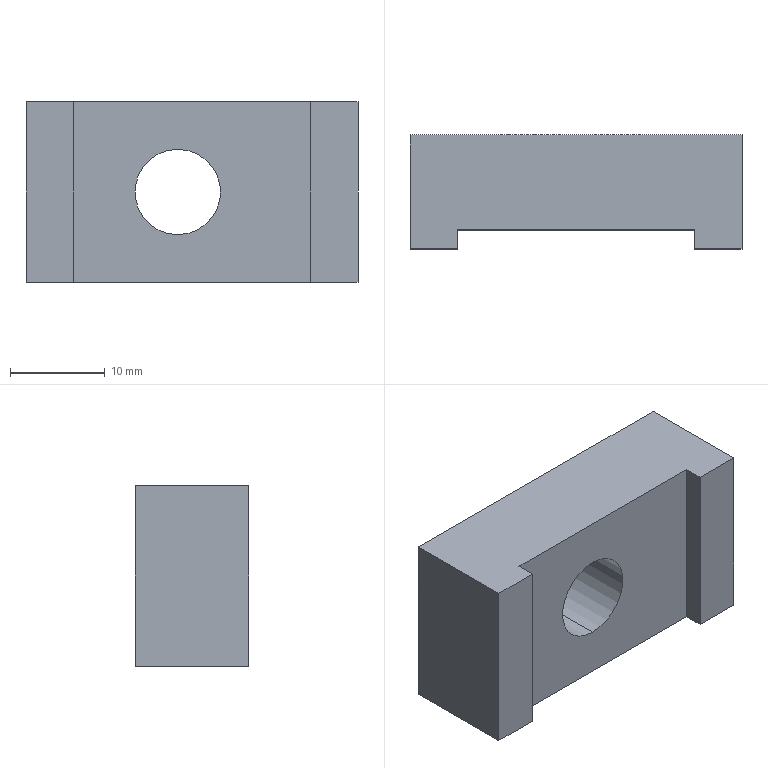Part | STEP file | OP10-023_clamp | 1 solid | 12 faces | box 35 x 12 x 19 mm | volume 6394 mm3 | plane 10 | cylinder 2 | commonest cylinder face diameters 9 x2
STEP:
#1=CARTESIAN_POINT('',(0.,0.,0.));
#2=DIRECTION('',(0.,0.,1.));
#3=DIRECTION('',(1.,0.,0.));
#4=AXIS2_PLACEMENT_3D('',#1,#2,#3);
#5=CARTESIAN_POINT('',(-1.5,-4.,14.));
#6=VERTEX_POINT('',#5);
#7=CARTESIAN_POINT('',(-1.5,6.,14.));
#8=VERTEX_POINT('',#7);
#9=CARTESIAN_POINT('',(-1.5,-13.,14.));
#10=DIRECTION('',(0.,1.,0.));
#11=VECTOR('',#10,1.);
#12=LINE('',#9,#11);
#13=CARTESIAN_POINT('',(-1.5,-13.,9.5));
#14=DIRECTION('',(0.,1.,0.));
#15=DIRECTION('',(0.,0.,1.));
#16=AXIS2_PLACEMENT_3D('',#13,#14,#15);
#17=CYLINDRICAL_SURFACE('',#16,4.5);
#18=CARTESIAN_POINT('',(6.283,0.));
#19=DIRECTION('',(0.,1.));
#20=VECTOR('',#19,1.);
#21=LINE('',#18,#20);
#22=(GEOMETRIC_REPRESENTATION_CONTEXT(2)PARAMETRIC_REPRESENTATION_CONTEXT()REPRESENTATION_CONTEXT('',''));
#23=DEFINITIONAL_REPRESENTATION('',(#21),#22);
#24=PCURVE('',#17,#23);
#25=CARTESIAN_POINT('',(-1.5,-13.,9.5));
#26=DIRECTION('',(0.,1.,0.));
#27=DIRECTION('',(0.,0.,1.));
#28=AXIS2_PLACEMENT_3D('',#25,#26,#27);
#29=CYLINDRICAL_SURFACE('',#28,4.5);
#30=CARTESIAN_POINT('',(0.,0.));
#31=DIRECTION('',(0.,1.));
#32=VECTOR('',#31,1.);
#33=LINE('',#30,#32);
#34=(GEOMETRIC_REPRESENTATION_CONTEXT(2)PARAMETRIC_REPRESENTATION_CONTEXT()REPRESENTATION_CONTEXT('',''));
#35=DEFINITIONAL_REPRESENTATION('',(#33),#34);
#36=PCURVE('',#29,#35);
#37=SURFACE_CURVE('',#12,(#24,#36),.PCURVE_S1.);
#38=EDGE_CURVE('',#6,#8,#37,.T.);
#39=ORIENTED_EDGE('',*,*,#38,.T.);
#40=CARTESIAN_POINT('',(-1.5,6.,5.));
#41=VERTEX_POINT('',#40);
#42=CARTESIAN_POINT('',(-1.5,6.,9.5));
#43=DIRECTION('',(0.,1.,0.));
#44=DIRECTION('',(0.,0.,1.));
#45=AXIS2_PLACEMENT_3D('',#42,#43,#44);
#46=CIRCLE('',#45,4.5);
#47=CARTESIAN_POINT('',(0.,19.));
#48=DIRECTION('',(1.,0.));
#49=VECTOR('',#48,1.);
#50=LINE('',#47,#49);
#51=(GEOMETRIC_REPRESENTATION_CONTEXT(2)PARAMETRIC_REPRESENTATION_CONTEXT()REPRESENTATION_CONTEXT('',''));
#52=DEFINITIONAL_REPRESENTATION('',(#50),#51);
#53=PCURVE('',#17,#52);
#54=CARTESIAN_POINT('',(-17.5,6.,19.));
#55=DIRECTION('',(0.,-1.,0.));
#56=DIRECTION('',(0.,0.,-1.));
#57=AXIS2_PLACEMENT_3D('',#54,#55,#56);
#58=PLANE('',#57);
#59=CARTESIAN_POINT('',(5.,16.));
#60=CARTESIAN_POINT('',(5.,23.794));
#61=CARTESIAN_POINT('',(11.75,19.897));
#62=CARTESIAN_POINT('',(18.5,16.));
#63=CARTESIAN_POINT('',(11.75,12.103));
#64=CARTESIAN_POINT('',(5.,8.206));
#65=CARTESIAN_POINT('',(5.,16.));
#66=(BOUNDED_CURVE()B_SPLINE_CURVE(2,(#59,#60,#61,#62,#63,#64,#65),.UNSPECIFIED.,.T.,.F.)B_SPLINE_CURVE_WITH_KNOTS((1,2,2,2,2,1),(-2.094,0.,2.094,4.189,6.283,8.378),.UNSPECIFIED.)CURVE()GEOMETRIC_REPRESENTATION_ITEM()RATIONAL_B_SPLINE_CURVE((1.,0.5,1.,0.5,1.,0.5,1.))REPRESENTATION_ITEM(''));
#67=(GEOMETRIC_REPRESENTATION_CONTEXT(2)PARAMETRIC_REPRESENTATION_CONTEXT()REPRESENTATION_CONTEXT('',''));
#68=DEFINITIONAL_REPRESENTATION('',(#66),#67);
#69=PCURVE('',#58,#68);
#70=SURFACE_CURVE('',#46,(#53,#69),.PCURVE_S1.);
#71=EDGE_CURVE('',#41,#8,#70,.T.);
#72=ORIENTED_EDGE('',*,*,#71,.F.);
#73=CARTESIAN_POINT('',(-1.5,-4.,5.));
#74=VERTEX_POINT('',#73);
#75=CARTESIAN_POINT('',(-1.5,-13.,5.));
#76=DIRECTION('',(0.,1.,0.));
#77=VECTOR('',#76,1.);
#78=LINE('',#75,#77);
#79=CARTESIAN_POINT('',(3.142,0.));
#80=DIRECTION('',(0.,1.));
#81=VECTOR('',#80,1.);
#82=LINE('',#79,#81);
#83=(GEOMETRIC_REPRESENTATION_CONTEXT(2)PARAMETRIC_REPRESENTATION_CONTEXT()REPRESENTATION_CONTEXT('',''));
#84=DEFINITIONAL_REPRESENTATION('',(#82),#83);
#85=PCURVE('',#17,#84);
#86=CARTESIAN_POINT('',(3.142,0.));
#87=DIRECTION('',(0.,1.));
#88=VECTOR('',#87,1.);
#89=LINE('',#86,#88);
#90=(GEOMETRIC_REPRESENTATION_CONTEXT(2)PARAMETRIC_REPRESENTATION_CONTEXT()REPRESENTATION_CONTEXT('',''));
#91=DEFINITIONAL_REPRESENTATION('',(#89),#90);
#92=PCURVE('',#29,#91);
#93=SURFACE_CURVE('',#78,(#85,#92),.PCURVE_S1.);
#94=EDGE_CURVE('',#74,#41,#93,.T.);
#95=ORIENTED_EDGE('',*,*,#94,.F.);
#96=CARTESIAN_POINT('',(-1.5,-4.,9.5));
#97=DIRECTION('',(0.,1.,0.));
#98=DIRECTION('',(-1.,0.,0.));
#99=AXIS2_PLACEMENT_3D('',#96,#97,#98);
#100=CIRCLE('',#99,4.5);
#101=CARTESIAN_POINT('',(-1.571,9.));
#102=DIRECTION('',(1.,0.));
#103=VECTOR('',#102,1.);
#104=LINE('',#101,#103);
#105=(GEOMETRIC_REPRESENTATION_CONTEXT(2)PARAMETRIC_REPRESENTATION_CONTEXT()REPRESENTATION_CONTEXT('',''));
#106=DEFINITIONAL_REPRESENTATION('',(#104),#105);
#107=PCURVE('',#17,#106);
#108=CARTESIAN_POINT('',(-12.5,-4.,19.));
#109=DIRECTION('',(0.,1.,0.));
#110=DIRECTION('',(-1.,0.,0.));
#111=AXIS2_PLACEMENT_3D('',#108,#109,#110);
#112=PLANE('',#111);
#113=CARTESIAN_POINT('',(-11.,-9.5));
#114=DIRECTION('',(1.,0.));
#115=AXIS2_PLACEMENT_2D('',#113,#114);
#116=CIRCLE('',#115,4.5);
#117=(GEOMETRIC_REPRESENTATION_CONTEXT(2)PARAMETRIC_REPRESENTATION_CONTEXT()REPRESENTATION_CONTEXT('',''));
#118=DEFINITIONAL_REPRESENTATION('',(#116),#117);
#119=PCURVE('',#112,#118);
#120=SURFACE_CURVE('',#100,(#107,#119),.PCURVE_S1.);
#121=EDGE_CURVE('',#74,#6,#120,.T.);
#122=ORIENTED_EDGE('',*,*,#121,.T.);
#123=EDGE_LOOP('',(#39,#72,#95,#122));
#124=FACE_BOUND('',#123,.F.);
#125=ADVANCED_FACE('',(#124),#17,.F.);
#126=CARTESIAN_POINT('',(12.5,-6.,0.));
#127=VERTEX_POINT('',#126);
#128=CARTESIAN_POINT('',(17.5,-6.,0.));
#129=VERTEX_POINT('',#128);
#130=CARTESIAN_POINT('',(12.5,-6.,0.));
#131=DIRECTION('',(1.,0.,0.));
#132=VECTOR('',#131,1.);
#133=LINE('',#130,#132);
#134=CARTESIAN_POINT('',(12.5,-6.,19.));
#135=DIRECTION('',(0.,1.,0.));
#136=DIRECTION('',(0.,0.,1.));
#137=AXIS2_PLACEMENT_3D('',#134,#135,#136);
#138=PLANE('',#137);
#139=CARTESIAN_POINT('',(-19.,0.));
#140=DIRECTION('',(0.,1.));
#141=VECTOR('',#140,1.);
#142=LINE('',#139,#141);
#143=(GEOMETRIC_REPRESENTATION_CONTEXT(2)PARAMETRIC_REPRESENTATION_CONTEXT()REPRESENTATION_CONTEXT('',''));
#144=DEFINITIONAL_REPRESENTATION('',(#142),#143);
#145=PCURVE('',#138,#144);
#146=CARTESIAN_POINT('',(0.,0.,0.));
#147=DIRECTION('',(0.,0.,-1.));
#148=DIRECTION('',(-1.,0.,0.));
#149=AXIS2_PLACEMENT_3D('',#146,#147,#148);
#150=PLANE('',#149);
#151=CARTESIAN_POINT('',(-12.5,-6.));
#152=DIRECTION('',(-1.,0.));
#153=VECTOR('',#152,1.);
#154=LINE('',#151,#153);
#155=(GEOMETRIC_REPRESENTATION_CONTEXT(2)PARAMETRIC_REPRESENTATION_CONTEXT()REPRESENTATION_CONTEXT('',''));
#156=DEFINITIONAL_REPRESENTATION('',(#154),#155);
#157=PCURVE('',#150,#156);
#158=SURFACE_CURVE('',#133,(#145,#157),.PCURVE_S1.);
#159=EDGE_CURVE('',#127,#129,#158,.T.);
#160=ORIENTED_EDGE('',*,*,#159,.T.);
#161=CARTESIAN_POINT('',(17.5,-6.,19.));
#162=VERTEX_POINT('',#161);
#163=CARTESIAN_POINT('',(17.5,-6.,19.));
#164=DIRECTION('',(0.,0.,-1.));
#165=VECTOR('',#164,1.);
#166=LINE('',#163,#165);
#167=CARTESIAN_POINT('',(0.,5.));
#168=DIRECTION('',(-1.,0.));
#169=VECTOR('',#168,1.);
#170=LINE('',#167,#169);
#171=(GEOMETRIC_REPRESENTATION_CONTEXT(2)PARAMETRIC_REPRESENTATION_CONTEXT()REPRESENTATION_CONTEXT('',''));
#172=DEFINITIONAL_REPRESENTATION('',(#170),#171);
#173=PCURVE('',#138,#172);
#174=CARTESIAN_POINT('',(17.5,6.,19.));
#175=DIRECTION('',(-1.,0.,0.));
#176=DIRECTION('',(0.,0.,1.));
#177=AXIS2_PLACEMENT_3D('',#174,#175,#176);
#178=PLANE('',#177);
#179=CARTESIAN_POINT('',(0.,-12.));
#180=DIRECTION('',(-1.,0.));
#181=VECTOR('',#180,1.);
#182=LINE('',#179,#181);
#183=(GEOMETRIC_REPRESENTATION_CONTEXT(2)PARAMETRIC_REPRESENTATION_CONTEXT()REPRESENTATION_CONTEXT('',''));
#184=DEFINITIONAL_REPRESENTATION('',(#182),#183);
#185=PCURVE('',#178,#184);
#186=SURFACE_CURVE('',#166,(#173,#185),.PCURVE_S1.);
#187=EDGE_CURVE('',#162,#129,#186,.T.);
#188=ORIENTED_EDGE('',*,*,#187,.F.);
#189=CARTESIAN_POINT('',(12.5,-6.,19.));
#190=VERTEX_POINT('',#189);
#191=CARTESIAN_POINT('',(12.5,-6.,19.));
#192=DIRECTION('',(1.,0.,0.));
#193=VECTOR('',#192,1.);
#194=LINE('',#191,#193);
#195=CARTESIAN_POINT('',(0.,0.));
#196=DIRECTION('',(0.,1.));
#197=VECTOR('',#196,1.);
#198=LINE('',#195,#197);
#199=(GEOMETRIC_REPRESENTATION_CONTEXT(2)PARAMETRIC_REPRESENTATION_CONTEXT()REPRESENTATION_CONTEXT('',''));
#200=DEFINITIONAL_REPRESENTATION('',(#198),#199);
#201=PCURVE('',#138,#200);
#202=CARTESIAN_POINT('',(0.,0.,19.));
#203=DIRECTION('',(0.,0.,-1.));
#204=DIRECTION('',(-1.,0.,0.));
#205=AXIS2_PLACEMENT_3D('',#202,#203,#204);
#206=PLANE('',#205);
#207=CARTESIAN_POINT('',(-12.5,-6.));
#208=DIRECTION('',(-1.,0.));
#209=VECTOR('',#208,1.);
#210=LINE('',#207,#209);
#211=(GEOMETRIC_REPRESENTATION_CONTEXT(2)PARAMETRIC_REPRESENTATION_CONTEXT()REPRESENTATION_CONTEXT('',''));
#212=DEFINITIONAL_REPRESENTATION('',(#210),#211);
#213=PCURVE('',#206,#212);
#214=SURFACE_CURVE('',#194,(#201,#213),.PCURVE_S1.);
#215=EDGE_CURVE('',#190,#162,#214,.T.);
#216=ORIENTED_EDGE('',*,*,#215,.F.);
#217=CARTESIAN_POINT('',(12.5,-6.,19.));
#218=DIRECTION('',(0.,0.,-1.));
#219=VECTOR('',#218,1.);
#220=LINE('',#217,#219);
#221=CARTESIAN_POINT('',(0.,0.));
#222=DIRECTION('',(-1.,0.));
#223=VECTOR('',#222,1.);
#224=LINE('',#221,#223);
#225=(GEOMETRIC_REPRESENTATION_CONTEXT(2)PARAMETRIC_REPRESENTATION_CONTEXT()REPRESENTATION_CONTEXT('',''));
#226=DEFINITIONAL_REPRESENTATION('',(#224),#225);
#227=PCURVE('',#138,#226);
#228=CARTESIAN_POINT('',(12.5,-6.,19.));
#229=DIRECTION('',(1.,0.,0.));
#230=DIRECTION('',(0.,0.,-1.));
#231=AXIS2_PLACEMENT_3D('',#228,#229,#230);
#232=PLANE('',#231);
#233=CARTESIAN_POINT('',(0.,0.));
#234=DIRECTION('',(1.,0.));
#235=VECTOR('',#234,1.);
#236=LINE('',#233,#235);
#237=(GEOMETRIC_REPRESENTATION_CONTEXT(2)PARAMETRIC_REPRESENTATION_CONTEXT()REPRESENTATION_CONTEXT('',''));
#238=DEFINITIONAL_REPRESENTATION('',(#236),#237);
#239=PCURVE('',#232,#238);
#240=SURFACE_CURVE('',#220,(#227,#239),.PCURVE_S1.);
#241=EDGE_CURVE('',#190,#127,#240,.T.);
#242=ORIENTED_EDGE('',*,*,#241,.T.);
#243=EDGE_LOOP('',(#160,#188,#216,#242));
#244=FACE_BOUND('',#243,.T.);
#245=ADVANCED_FACE('',(#244),#138,.F.);
#246=CARTESIAN_POINT('',(17.5,6.,0.));
#247=VERTEX_POINT('',#246);
#248=CARTESIAN_POINT('',(17.5,6.,0.));
#249=DIRECTION('',(0.,1.,0.));
#250=VECTOR('',#249,1.);
#251=LINE('',#248,#250);
#252=CARTESIAN_POINT('',(-19.,0.));
#253=DIRECTION('',(0.,1.));
#254=VECTOR('',#253,1.);
#255=LINE('',#252,#254);
#256=(GEOMETRIC_REPRESENTATION_CONTEXT(2)PARAMETRIC_REPRESENTATION_CONTEXT()REPRESENTATION_CONTEXT('',''));
#257=DEFINITIONAL_REPRESENTATION('',(#255),#256);
#258=PCURVE('',#178,#257);
#259=CARTESIAN_POINT('',(-17.5,6.));
#260=DIRECTION('',(0.,1.));
#261=VECTOR('',#260,1.);
#262=LINE('',#259,#261);
#263=(GEOMETRIC_REPRESENTATION_CONTEXT(2)PARAMETRIC_REPRESENTATION_CONTEXT()REPRESENTATION_CONTEXT('',''));
#264=DEFINITIONAL_REPRESENTATION('',(#262),#263);
#265=PCURVE('',#150,#264);
#266=SURFACE_CURVE('',#251,(#258,#265),.PCURVE_S1.);
#267=EDGE_CURVE('',#129,#247,#266,.T.);
#268=ORIENTED_EDGE('',*,*,#267,.T.);
#269=CARTESIAN_POINT('',(17.5,6.,19.));
#270=VERTEX_POINT('',#269);
#271=CARTESIAN_POINT('',(17.5,6.,19.));
#272=DIRECTION('',(0.,0.,-1.));
#273=VECTOR('',#272,1.);
#274=LINE('',#271,#273);
#275=CARTESIAN_POINT('',(0.,0.));
#276=DIRECTION('',(-1.,0.));
#277=VECTOR('',#276,1.);
#278=LINE('',#275,#277);
#279=(GEOMETRIC_REPRESENTATION_CONTEXT(2)PARAMETRIC_REPRESENTATION_CONTEXT()REPRESENTATION_CONTEXT('',''));
#280=DEFINITIONAL_REPRESENTATION('',(#278),#279);
#281=PCURVE('',#178,#280);
#282=CARTESIAN_POINT('',(0.,35.));
#283=DIRECTION('',(1.,0.));
#284=VECTOR('',#283,1.);
#285=LINE('',#282,#284);
#286=(GEOMETRIC_REPRESENTATION_CONTEXT(2)PARAMETRIC_REPRESENTATION_CONTEXT()REPRESENTATION_CONTEXT('',''));
#287=DEFINITIONAL_REPRESENTATION('',(#285),#286);
#288=PCURVE('',#58,#287);
#289=SURFACE_CURVE('',#274,(#281,#288),.PCURVE_S1.);
#290=EDGE_CURVE('',#270,#247,#289,.T.);
#291=ORIENTED_EDGE('',*,*,#290,.F.);
#292=CARTESIAN_POINT('',(17.5,6.,19.));
#293=DIRECTION('',(0.,1.,0.));
#294=VECTOR('',#293,1.);
#295=LINE('',#292,#294);
#296=CARTESIAN_POINT('',(0.,0.));
#297=DIRECTION('',(0.,1.));
#298=VECTOR('',#297,1.);
#299=LINE('',#296,#298);
#300=(GEOMETRIC_REPRESENTATION_CONTEXT(2)PARAMETRIC_REPRESENTATION_CONTEXT()REPRESENTATION_CONTEXT('',''));
#301=DEFINITIONAL_REPRESENTATION('',(#299),#300);
#302=PCURVE('',#178,#301);
#303=CARTESIAN_POINT('',(-17.5,6.));
#304=DIRECTION('',(0.,1.));
#305=VECTOR('',#304,1.);
#306=LINE('',#303,#305);
#307=(GEOMETRIC_REPRESENTATION_CONTEXT(2)PARAMETRIC_REPRESENTATION_CONTEXT()REPRESENTATION_CONTEXT('',''));
#308=DEFINITIONAL_REPRESENTATION('',(#306),#307);
#309=PCURVE('',#206,#308);
#310=SURFACE_CURVE('',#295,(#302,#309),.PCURVE_S1.);
#311=EDGE_CURVE('',#162,#270,#310,.T.);
#312=ORIENTED_EDGE('',*,*,#311,.F.);
#313=ORIENTED_EDGE('',*,*,#187,.T.);
#314=EDGE_LOOP('',(#268,#291,#312,#313));
#315=FACE_BOUND('',#314,.T.);
#316=ADVANCED_FACE('',(#315),#178,.F.);
#317=CARTESIAN_POINT('',(-1.5,6.,9.5));
#318=DIRECTION('',(0.,1.,0.));
#319=DIRECTION('',(0.,0.,1.));
#320=AXIS2_PLACEMENT_3D('',#317,#318,#319);
#321=CIRCLE('',#320,4.5);
#322=CARTESIAN_POINT('',(5.,16.));
#323=CARTESIAN_POINT('',(5.,23.794));
#324=CARTESIAN_POINT('',(11.75,19.897));
#325=CARTESIAN_POINT('',(18.5,16.));
#326=CARTESIAN_POINT('',(11.75,12.103));
#327=CARTESIAN_POINT('',(5.,8.206));
#328=CARTESIAN_POINT('',(5.,16.));
#329=(BOUNDED_CURVE()B_SPLINE_CURVE(2,(#322,#323,#324,#325,#326,#327,#328),.UNSPECIFIED.,.T.,.F.)B_SPLINE_CURVE_WITH_KNOTS((1,2,2,2,2,1),(-2.094,0.,2.094,4.189,6.283,8.378),.UNSPECIFIED.)CURVE()GEOMETRIC_REPRESENTATION_ITEM()RATIONAL_B_SPLINE_CURVE((1.,0.5,1.,0.5,1.,0.5,1.))REPRESENTATION_ITEM(''));
#330=(GEOMETRIC_REPRESENTATION_CONTEXT(2)PARAMETRIC_REPRESENTATION_CONTEXT()REPRESENTATION_CONTEXT('',''));
#331=DEFINITIONAL_REPRESENTATION('',(#329),#330);
#332=PCURVE('',#58,#331);
#333=CARTESIAN_POINT('',(0.,19.));
#334=DIRECTION('',(1.,0.));
#335=VECTOR('',#334,1.);
#336=LINE('',#333,#335);
#337=(GEOMETRIC_REPRESENTATION_CONTEXT(2)PARAMETRIC_REPRESENTATION_CONTEXT()REPRESENTATION_CONTEXT('',''));
#338=DEFINITIONAL_REPRESENTATION('',(#336),#337);
#339=PCURVE('',#29,#338);
#340=SURFACE_CURVE('',#321,(#332,#339),.PCURVE_S1.);
#341=EDGE_CURVE('',#8,#41,#340,.T.);
#342=ORIENTED_EDGE('',*,*,#341,.F.);
#343=ORIENTED_EDGE('',*,*,#71,.F.);
#344=EDGE_LOOP('',(#342,#343));
#345=FACE_BOUND('',#344,.T.);
#346=CARTESIAN_POINT('',(-17.5,6.,0.));
#347=VERTEX_POINT('',#346);
#348=CARTESIAN_POINT('',(-17.5,6.,0.));
#349=DIRECTION('',(-1.,0.,0.));
#350=VECTOR('',#349,1.);
#351=LINE('',#348,#350);
#352=CARTESIAN_POINT('',(19.,0.));
#353=DIRECTION('',(0.,-1.));
#354=VECTOR('',#353,1.);
#355=LINE('',#352,#354);
#356=(GEOMETRIC_REPRESENTATION_CONTEXT(2)PARAMETRIC_REPRESENTATION_CONTEXT()REPRESENTATION_CONTEXT('',''));
#357=DEFINITIONAL_REPRESENTATION('',(#355),#356);
#358=PCURVE('',#58,#357);
#359=CARTESIAN_POINT('',(17.5,6.));
#360=DIRECTION('',(1.,0.));
#361=VECTOR('',#360,1.);
#362=LINE('',#359,#361);
#363=(GEOMETRIC_REPRESENTATION_CONTEXT(2)PARAMETRIC_REPRESENTATION_CONTEXT()REPRESENTATION_CONTEXT('',''));
#364=DEFINITIONAL_REPRESENTATION('',(#362),#363);
#365=PCURVE('',#150,#364);
#366=SURFACE_CURVE('',#351,(#358,#365),.PCURVE_S1.);
#367=EDGE_CURVE('',#247,#347,#366,.T.);
#368=ORIENTED_EDGE('',*,*,#367,.T.);
#369=CARTESIAN_POINT('',(-17.5,6.,19.));
#370=VERTEX_POINT('',#369);
#371=CARTESIAN_POINT('',(-17.5,6.,19.));
#372=DIRECTION('',(0.,0.,-1.));
#373=VECTOR('',#372,1.);
#374=LINE('',#371,#373);
#375=CARTESIAN_POINT('',(0.,0.));
#376=DIRECTION('',(1.,0.));
#377=VECTOR('',#376,1.);
#378=LINE('',#375,#377);
#379=(GEOMETRIC_REPRESENTATION_CONTEXT(2)PARAMETRIC_REPRESENTATION_CONTEXT()REPRESENTATION_CONTEXT('',''));
#380=DEFINITIONAL_REPRESENTATION('',(#378),#379);
#381=PCURVE('',#58,#380);
#382=CARTESIAN_POINT('',(-17.5,6.,19.));
#383=DIRECTION('',(1.,0.,0.));
#384=DIRECTION('',(0.,0.,-1.));
#385=AXIS2_PLACEMENT_3D('',#382,#383,#384);
#386=PLANE('',#385);
#387=CARTESIAN_POINT('',(0.,0.));
#388=DIRECTION('',(1.,0.));
#389=VECTOR('',#388,1.);
#390=LINE('',#387,#389);
#391=(GEOMETRIC_REPRESENTATION_CONTEXT(2)PARAMETRIC_REPRESENTATION_CONTEXT()REPRESENTATION_CONTEXT('',''));
#392=DEFINITIONAL_REPRESENTATION('',(#390),#391);
#393=PCURVE('',#386,#392);
#394=SURFACE_CURVE('',#374,(#381,#393),.PCURVE_S1.);
#395=EDGE_CURVE('',#370,#347,#394,.T.);
#396=ORIENTED_EDGE('',*,*,#395,.F.);
#397=CARTESIAN_POINT('',(-17.5,6.,19.));
#398=DIRECTION('',(-1.,0.,0.));
#399=VECTOR('',#398,1.);
#400=LINE('',#397,#399);
#401=CARTESIAN_POINT('',(0.,0.));
#402=DIRECTION('',(0.,-1.));
#403=VECTOR('',#402,1.);
#404=LINE('',#401,#403);
#405=(GEOMETRIC_REPRESENTATION_CONTEXT(2)PARAMETRIC_REPRESENTATION_CONTEXT()REPRESENTATION_CONTEXT('',''));
#406=DEFINITIONAL_REPRESENTATION('',(#404),#405);
#407=PCURVE('',#58,#406);
#408=CARTESIAN_POINT('',(17.5,6.));
#409=DIRECTION('',(1.,0.));
#410=VECTOR('',#409,1.);
#411=LINE('',#408,#410);
#412=(GEOMETRIC_REPRESENTATION_CONTEXT(2)PARAMETRIC_REPRESENTATION_CONTEXT()REPRESENTATION_CONTEXT('',''));
#413=DEFINITIONAL_REPRESENTATION('',(#411),#412);
#414=PCURVE('',#206,#413);
#415=SURFACE_CURVE('',#400,(#407,#414),.PCURVE_S1.);
#416=EDGE_CURVE('',#270,#370,#415,.T.);
#417=ORIENTED_EDGE('',*,*,#416,.F.);
#418=ORIENTED_EDGE('',*,*,#290,.T.);
#419=EDGE_LOOP('',(#368,#396,#417,#418));
#420=FACE_BOUND('',#419,.T.);
#421=ADVANCED_FACE('',(#345,#420),#58,.F.);
#422=CARTESIAN_POINT('',(-17.5,-6.,0.));
#423=VERTEX_POINT('',#422);
#424=CARTESIAN_POINT('',(-17.5,6.,0.));
#425=DIRECTION('',(0.,-1.,0.));
#426=VECTOR('',#425,1.);
#427=LINE('',#424,#426);
#428=CARTESIAN_POINT('',(19.,0.));
#429=DIRECTION('',(0.,-1.));
#430=VECTOR('',#429,1.);
#431=LINE('',#428,#430);
#432=(GEOMETRIC_REPRESENTATION_CONTEXT(2)PARAMETRIC_REPRESENTATION_CONTEXT()REPRESENTATION_CONTEXT('',''));
#433=DEFINITIONAL_REPRESENTATION('',(#431),#432);
#434=PCURVE('',#386,#433);
#435=CARTESIAN_POINT('',(17.5,6.));
#436=DIRECTION('',(0.,-1.));
#437=VECTOR('',#436,1.);
#438=LINE('',#435,#437);
#439=(GEOMETRIC_REPRESENTATION_CONTEXT(2)PARAMETRIC_REPRESENTATION_CONTEXT()REPRESENTATION_CONTEXT('',''));
#440=DEFINITIONAL_REPRESENTATION('',(#438),#439);
#441=PCURVE('',#150,#440);
#442=SURFACE_CURVE('',#427,(#434,#441),.PCURVE_S1.);
#443=EDGE_CURVE('',#347,#423,#442,.T.);
#444=ORIENTED_EDGE('',*,*,#443,.T.);
#445=CARTESIAN_POINT('',(-17.5,-6.,19.));
#446=VERTEX_POINT('',#445);
#447=CARTESIAN_POINT('',(-17.5,-6.,19.));
#448=DIRECTION('',(0.,0.,-1.));
#449=VECTOR('',#448,1.);
#450=LINE('',#447,#449);
#451=CARTESIAN_POINT('',(0.,-12.));
#452=DIRECTION('',(1.,0.));
#453=VECTOR('',#452,1.);
#454=LINE('',#451,#453);
#455=(GEOMETRIC_REPRESENTATION_CONTEXT(2)PARAMETRIC_REPRESENTATION_CONTEXT()REPRESENTATION_CONTEXT('',''));
#456=DEFINITIONAL_REPRESENTATION('',(#454),#455);
#457=PCURVE('',#386,#456);
#458=CARTESIAN_POINT('',(-17.5,-6.,19.));
#459=DIRECTION('',(0.,1.,0.));
#460=DIRECTION('',(-1.,0.,0.));
#461=AXIS2_PLACEMENT_3D('',#458,#459,#460);
#462=PLANE('',#461);
#463=CARTESIAN_POINT('',(0.,0.));
#464=DIRECTION('',(0.,-1.));
#465=VECTOR('',#464,1.);
#466=LINE('',#463,#465);
#467=(GEOMETRIC_REPRESENTATION_CONTEXT(2)PARAMETRIC_REPRESENTATION_CONTEXT()REPRESENTATION_CONTEXT('',''));
#468=DEFINITIONAL_REPRESENTATION('',(#466),#467);
#469=PCURVE('',#462,#468);
#470=SURFACE_CURVE('',#450,(#457,#469),.PCURVE_S1.);
#471=EDGE_CURVE('',#446,#423,#470,.T.);
#472=ORIENTED_EDGE('',*,*,#471,.F.);
#473=CARTESIAN_POINT('',(-17.5,6.,19.));
#474=DIRECTION('',(0.,-1.,0.));
#475=VECTOR('',#474,1.);
#476=LINE('',#473,#475);
#477=CARTESIAN_POINT('',(0.,0.));
#478=DIRECTION('',(0.,-1.));
#479=VECTOR('',#478,1.);
#480=LINE('',#477,#479);
#481=(GEOMETRIC_REPRESENTATION_CONTEXT(2)PARAMETRIC_REPRESENTATION_CONTEXT()REPRESENTATION_CONTEXT('',''));
#482=DEFINITIONAL_REPRESENTATION('',(#480),#481);
#483=PCURVE('',#386,#482);
#484=CARTESIAN_POINT('',(17.5,6.));
#485=DIRECTION('',(0.,-1.));
#486=VECTOR('',#485,1.);
#487=LINE('',#484,#486);
#488=(GEOMETRIC_REPRESENTATION_CONTEXT(2)PARAMETRIC_REPRESENTATION_CONTEXT()REPRESENTATION_CONTEXT('',''));
#489=DEFINITIONAL_REPRESENTATION('',(#487),#488);
#490=PCURVE('',#206,#489);
#491=SURFACE_CURVE('',#476,(#483,#490),.PCURVE_S1.);
#492=EDGE_CURVE('',#370,#446,#491,.T.);
#493=ORIENTED_EDGE('',*,*,#492,.F.);
#494=ORIENTED_EDGE('',*,*,#395,.T.);
#495=EDGE_LOOP('',(#444,#472,#493,#494));
#496=FACE_BOUND('',#495,.T.);
#497=ADVANCED_FACE('',(#496),#386,.F.);
#498=CARTESIAN_POINT('',(-12.5,-6.,0.));
#499=VERTEX_POINT('',#498);
#500=CARTESIAN_POINT('',(-17.5,-6.,0.));
#501=DIRECTION('',(1.,0.,0.));
#502=VECTOR('',#501,1.);
#503=LINE('',#500,#502);
#504=CARTESIAN_POINT('',(0.,-19.));
#505=DIRECTION('',(-1.,0.));
#506=VECTOR('',#505,1.);
#507=LINE('',#504,#506);
#508=(GEOMETRIC_REPRESENTATION_CONTEXT(2)PARAMETRIC_REPRESENTATION_CONTEXT()REPRESENTATION_CONTEXT('',''));
#509=DEFINITIONAL_REPRESENTATION('',(#507),#508);
#510=PCURVE('',#462,#509);
#511=CARTESIAN_POINT('',(17.5,-6.));
#512=DIRECTION('',(-1.,0.));
#513=VECTOR('',#512,1.);
#514=LINE('',#511,#513);
#515=(GEOMETRIC_REPRESENTATION_CONTEXT(2)PARAMETRIC_REPRESENTATION_CONTEXT()REPRESENTATION_CONTEXT('',''));
#516=DEFINITIONAL_REPRESENTATION('',(#514),#515);
#517=PCURVE('',#150,#516);
#518=SURFACE_CURVE('',#503,(#510,#517),.PCURVE_S1.);
#519=EDGE_CURVE('',#423,#499,#518,.T.);
#520=ORIENTED_EDGE('',*,*,#519,.T.);
#521=CARTESIAN_POINT('',(-12.5,-6.,19.));
#522=VERTEX_POINT('',#521);
#523=CARTESIAN_POINT('',(-12.5,-6.,19.));
#524=DIRECTION('',(0.,0.,-1.));
#525=VECTOR('',#524,1.);
#526=LINE('',#523,#525);
#527=CARTESIAN_POINT('',(-5.,0.));
#528=DIRECTION('',(0.,-1.));
#529=VECTOR('',#528,1.);
#530=LINE('',#527,#529);
#531=(GEOMETRIC_REPRESENTATION_CONTEXT(2)PARAMETRIC_REPRESENTATION_CONTEXT()REPRESENTATION_CONTEXT('',''));
#532=DEFINITIONAL_REPRESENTATION('',(#530),#531);
#533=PCURVE('',#462,#532);
#534=CARTESIAN_POINT('',(-12.5,-6.,19.));
#535=DIRECTION('',(-1.,0.,0.));
#536=DIRECTION('',(0.,0.,1.));
#537=AXIS2_PLACEMENT_3D('',#534,#535,#536);
#538=PLANE('',#537);
#539=CARTESIAN_POINT('',(0.,0.));
#540=DIRECTION('',(-1.,0.));
#541=VECTOR('',#540,1.);
#542=LINE('',#539,#541);
#543=(GEOMETRIC_REPRESENTATION_CONTEXT(2)PARAMETRIC_REPRESENTATION_CONTEXT()REPRESENTATION_CONTEXT('',''));
#544=DEFINITIONAL_REPRESENTATION('',(#542),#543);
#545=PCURVE('',#538,#544);
#546=SURFACE_CURVE('',#526,(#533,#545),.PCURVE_S1.);
#547=EDGE_CURVE('',#522,#499,#546,.T.);
#548=ORIENTED_EDGE('',*,*,#547,.F.);
#549=CARTESIAN_POINT('',(-17.5,-6.,19.));
#550=DIRECTION('',(1.,0.,0.));
#551=VECTOR('',#550,1.);
#552=LINE('',#549,#551);
#553=CARTESIAN_POINT('',(0.,0.));
#554=DIRECTION('',(-1.,0.));
#555=VECTOR('',#554,1.);
#556=LINE('',#553,#555);
#557=(GEOMETRIC_REPRESENTATION_CONTEXT(2)PARAMETRIC_REPRESENTATION_CONTEXT()REPRESENTATION_CONTEXT('',''));
#558=DEFINITIONAL_REPRESENTATION('',(#556),#557);
#559=PCURVE('',#462,#558);
#560=CARTESIAN_POINT('',(17.5,-6.));
#561=DIRECTION('',(-1.,0.));
#562=VECTOR('',#561,1.);
#563=LINE('',#560,#562);
#564=(GEOMETRIC_REPRESENTATION_CONTEXT(2)PARAMETRIC_REPRESENTATION_CONTEXT()REPRESENTATION_CONTEXT('',''));
#565=DEFINITIONAL_REPRESENTATION('',(#563),#564);
#566=PCURVE('',#206,#565);
#567=SURFACE_CURVE('',#552,(#559,#566),.PCURVE_S1.);
#568=EDGE_CURVE('',#446,#522,#567,.T.);
#569=ORIENTED_EDGE('',*,*,#568,.F.);
#570=ORIENTED_EDGE('',*,*,#471,.T.);
#571=EDGE_LOOP('',(#520,#548,#569,#570));
#572=FACE_BOUND('',#571,.T.);
#573=ADVANCED_FACE('',(#572),#462,.F.);
#574=CARTESIAN_POINT('',(-12.5,-4.,0.));
#575=VERTEX_POINT('',#574);
#576=CARTESIAN_POINT('',(-12.5,-6.,0.));
#577=DIRECTION('',(0.,1.,0.));
#578=VECTOR('',#577,1.);
#579=LINE('',#576,#578);
#580=CARTESIAN_POINT('',(-19.,0.));
#581=DIRECTION('',(0.,1.));
#582=VECTOR('',#581,1.);
#583=LINE('',#580,#582);
#584=(GEOMETRIC_REPRESENTATION_CONTEXT(2)PARAMETRIC_REPRESENTATION_CONTEXT()REPRESENTATION_CONTEXT('',''));
#585=DEFINITIONAL_REPRESENTATION('',(#583),#584);
#586=PCURVE('',#538,#585);
#587=CARTESIAN_POINT('',(12.5,-6.));
#588=DIRECTION('',(0.,1.));
#589=VECTOR('',#588,1.);
#590=LINE('',#587,#589);
#591=(GEOMETRIC_REPRESENTATION_CONTEXT(2)PARAMETRIC_REPRESENTATION_CONTEXT()REPRESENTATION_CONTEXT('',''));
#592=DEFINITIONAL_REPRESENTATION('',(#590),#591);
#593=PCURVE('',#150,#592);
#594=SURFACE_CURVE('',#579,(#586,#593),.PCURVE_S1.);
#595=EDGE_CURVE('',#499,#575,#594,.T.);
#596=ORIENTED_EDGE('',*,*,#595,.T.);
#597=CARTESIAN_POINT('',(-12.5,-4.,19.));
#598=VERTEX_POINT('',#597);
#599=CARTESIAN_POINT('',(-12.5,-4.,19.));
#600=DIRECTION('',(0.,0.,-1.));
#601=VECTOR('',#600,1.);
#602=LINE('',#599,#601);
#603=CARTESIAN_POINT('',(0.,2.));
#604=DIRECTION('',(-1.,0.));
#605=VECTOR('',#604,1.);
#606=LINE('',#603,#605);
#607=(GEOMETRIC_REPRESENTATION_CONTEXT(2)PARAMETRIC_REPRESENTATION_CONTEXT()REPRESENTATION_CONTEXT('',''));
#608=DEFINITIONAL_REPRESENTATION('',(#606),#607);
#609=PCURVE('',#538,#608);
#610=CARTESIAN_POINT('',(0.,0.));
#611=DIRECTION('',(0.,-1.));
#612=VECTOR('',#611,1.);
#613=LINE('',#610,#612);
#614=(GEOMETRIC_REPRESENTATION_CONTEXT(2)PARAMETRIC_REPRESENTATION_CONTEXT()REPRESENTATION_CONTEXT('',''));
#615=DEFINITIONAL_REPRESENTATION('',(#613),#614);
#616=PCURVE('',#112,#615);
#617=SURFACE_CURVE('',#602,(#609,#616),.PCURVE_S1.);
#618=EDGE_CURVE('',#598,#575,#617,.T.);
#619=ORIENTED_EDGE('',*,*,#618,.F.);
#620=CARTESIAN_POINT('',(-12.5,-6.,19.));
#621=DIRECTION('',(0.,1.,0.));
#622=VECTOR('',#621,1.);
#623=LINE('',#620,#622);
#624=CARTESIAN_POINT('',(0.,0.));
#625=DIRECTION('',(0.,1.));
#626=VECTOR('',#625,1.);
#627=LINE('',#624,#626);
#628=(GEOMETRIC_REPRESENTATION_CONTEXT(2)PARAMETRIC_REPRESENTATION_CONTEXT()REPRESENTATION_CONTEXT('',''));
#629=DEFINITIONAL_REPRESENTATION('',(#627),#628);
#630=PCURVE('',#538,#629);
#631=CARTESIAN_POINT('',(12.5,-6.));
#632=DIRECTION('',(0.,1.));
#633=VECTOR('',#632,1.);
#634=LINE('',#631,#633);
#635=(GEOMETRIC_REPRESENTATION_CONTEXT(2)PARAMETRIC_REPRESENTATION_CONTEXT()REPRESENTATION_CONTEXT('',''));
#636=DEFINITIONAL_REPRESENTATION('',(#634),#635);
#637=PCURVE('',#206,#636);
#638=SURFACE_CURVE('',#623,(#630,#637),.PCURVE_S1.);
#639=EDGE_CURVE('',#522,#598,#638,.T.);
#640=ORIENTED_EDGE('',*,*,#639,.F.);
#641=ORIENTED_EDGE('',*,*,#547,.T.);
#642=EDGE_LOOP('',(#596,#619,#640,#641));
#643=FACE_BOUND('',#642,.T.);
#644=ADVANCED_FACE('',(#643),#538,.F.);
#645=CARTESIAN_POINT('',(-1.5,-4.,9.5));
#646=DIRECTION('',(0.,1.,0.));
#647=DIRECTION('',(-1.,0.,0.));
#648=AXIS2_PLACEMENT_3D('',#645,#646,#647);
#649=CIRCLE('',#648,4.5);
#650=CARTESIAN_POINT('',(-11.,-9.5));
#651=DIRECTION('',(1.,0.));
#652=AXIS2_PLACEMENT_2D('',#650,#651);
#653=CIRCLE('',#652,4.5);
#654=(GEOMETRIC_REPRESENTATION_CONTEXT(2)PARAMETRIC_REPRESENTATION_CONTEXT()REPRESENTATION_CONTEXT('',''));
#655=DEFINITIONAL_REPRESENTATION('',(#653),#654);
#656=PCURVE('',#112,#655);
#657=CARTESIAN_POINT('',(-1.571,9.));
#658=DIRECTION('',(1.,0.));
#659=VECTOR('',#658,1.);
#660=LINE('',#657,#659);
#661=(GEOMETRIC_REPRESENTATION_CONTEXT(2)PARAMETRIC_REPRESENTATION_CONTEXT()REPRESENTATION_CONTEXT('',''));
#662=DEFINITIONAL_REPRESENTATION('',(#660),#661);
#663=PCURVE('',#29,#662);
#664=SURFACE_CURVE('',#649,(#656,#663),.PCURVE_S1.);
#665=EDGE_CURVE('',#6,#74,#664,.T.);
#666=ORIENTED_EDGE('',*,*,#665,.T.);
#667=ORIENTED_EDGE('',*,*,#121,.T.);
#668=EDGE_LOOP('',(#666,#667));
#669=FACE_BOUND('',#668,.T.);
#670=CARTESIAN_POINT('',(12.5,-4.,0.));
#671=VERTEX_POINT('',#670);
#672=CARTESIAN_POINT('',(-12.5,-4.,0.));
#673=DIRECTION('',(1.,0.,0.));
#674=VECTOR('',#673,1.);
#675=LINE('',#672,#674);
#676=CARTESIAN_POINT('',(0.,-19.));
#677=DIRECTION('',(-1.,0.));
#678=VECTOR('',#677,1.);
#679=LINE('',#676,#678);
#680=(GEOMETRIC_REPRESENTATION_CONTEXT(2)PARAMETRIC_REPRESENTATION_CONTEXT()REPRESENTATION_CONTEXT('',''));
#681=DEFINITIONAL_REPRESENTATION('',(#679),#680);
#682=PCURVE('',#112,#681);
#683=CARTESIAN_POINT('',(12.5,-4.));
#684=DIRECTION('',(-1.,0.));
#685=VECTOR('',#684,1.);
#686=LINE('',#683,#685);
#687=(GEOMETRIC_REPRESENTATION_CONTEXT(2)PARAMETRIC_REPRESENTATION_CONTEXT()REPRESENTATION_CONTEXT('',''));
#688=DEFINITIONAL_REPRESENTATION('',(#686),#687);
#689=PCURVE('',#150,#688);
#690=SURFACE_CURVE('',#675,(#682,#689),.PCURVE_S1.);
#691=EDGE_CURVE('',#575,#671,#690,.T.);
#692=ORIENTED_EDGE('',*,*,#691,.T.);
#693=CARTESIAN_POINT('',(12.5,-4.,19.));
#694=VERTEX_POINT('',#693);
#695=CARTESIAN_POINT('',(12.5,-4.,19.));
#696=DIRECTION('',(0.,0.,-1.));
#697=VECTOR('',#696,1.);
#698=LINE('',#695,#697);
#699=CARTESIAN_POINT('',(-25.,0.));
#700=DIRECTION('',(0.,-1.));
#701=VECTOR('',#700,1.);
#702=LINE('',#699,#701);
#703=(GEOMETRIC_REPRESENTATION_CONTEXT(2)PARAMETRIC_REPRESENTATION_CONTEXT()REPRESENTATION_CONTEXT('',''));
#704=DEFINITIONAL_REPRESENTATION('',(#702),#703);
#705=PCURVE('',#112,#704);
#706=CARTESIAN_POINT('',(0.,2.));
#707=DIRECTION('',(1.,0.));
#708=VECTOR('',#707,1.);
#709=LINE('',#706,#708);
#710=(GEOMETRIC_REPRESENTATION_CONTEXT(2)PARAMETRIC_REPRESENTATION_CONTEXT()REPRESENTATION_CONTEXT('',''));
#711=DEFINITIONAL_REPRESENTATION('',(#709),#710);
#712=PCURVE('',#232,#711);
#713=SURFACE_CURVE('',#698,(#705,#712),.PCURVE_S1.);
#714=EDGE_CURVE('',#694,#671,#713,.T.);
#715=ORIENTED_EDGE('',*,*,#714,.F.);
#716=CARTESIAN_POINT('',(-12.5,-4.,19.));
#717=DIRECTION('',(1.,0.,0.));
#718=VECTOR('',#717,1.);
#719=LINE('',#716,#718);
#720=CARTESIAN_POINT('',(0.,0.));
#721=DIRECTION('',(-1.,0.));
#722=VECTOR('',#721,1.);
#723=LINE('',#720,#722);
#724=(GEOMETRIC_REPRESENTATION_CONTEXT(2)PARAMETRIC_REPRESENTATION_CONTEXT()REPRESENTATION_CONTEXT('',''));
#725=DEFINITIONAL_REPRESENTATION('',(#723),#724);
#726=PCURVE('',#112,#725);
#727=CARTESIAN_POINT('',(12.5,-4.));
#728=DIRECTION('',(-1.,0.));
#729=VECTOR('',#728,1.);
#730=LINE('',#727,#729);
#731=(GEOMETRIC_REPRESENTATION_CONTEXT(2)PARAMETRIC_REPRESENTATION_CONTEXT()REPRESENTATION_CONTEXT('',''));
#732=DEFINITIONAL_REPRESENTATION('',(#730),#731);
#733=PCURVE('',#206,#732);
#734=SURFACE_CURVE('',#719,(#726,#733),.PCURVE_S1.);
#735=EDGE_CURVE('',#598,#694,#734,.T.);
#736=ORIENTED_EDGE('',*,*,#735,.F.);
#737=ORIENTED_EDGE('',*,*,#618,.T.);
#738=EDGE_LOOP('',(#692,#715,#736,#737));
#739=FACE_BOUND('',#738,.T.);
#740=ADVANCED_FACE('',(#669,#739),#112,.F.);
#741=CARTESIAN_POINT('',(12.5,-6.,0.));
#742=DIRECTION('',(0.,-1.,0.));
#743=VECTOR('',#742,1.);
#744=LINE('',#741,#743);
#745=CARTESIAN_POINT('',(19.,0.));
#746=DIRECTION('',(0.,-1.));
#747=VECTOR('',#746,1.);
#748=LINE('',#745,#747);
#749=(GEOMETRIC_REPRESENTATION_CONTEXT(2)PARAMETRIC_REPRESENTATION_CONTEXT()REPRESENTATION_CONTEXT('',''));
#750=DEFINITIONAL_REPRESENTATION('',(#748),#749);
#751=PCURVE('',#232,#750);
#752=CARTESIAN_POINT('',(-12.5,-6.));
#753=DIRECTION('',(0.,-1.));
#754=VECTOR('',#753,1.);
#755=LINE('',#752,#754);
#756=(GEOMETRIC_REPRESENTATION_CONTEXT(2)PARAMETRIC_REPRESENTATION_CONTEXT()REPRESENTATION_CONTEXT('',''));
#757=DEFINITIONAL_REPRESENTATION('',(#755),#756);
#758=PCURVE('',#150,#757);
#759=SURFACE_CURVE('',#744,(#751,#758),.PCURVE_S1.);
#760=EDGE_CURVE('',#671,#127,#759,.T.);
#761=ORIENTED_EDGE('',*,*,#760,.T.);
#762=ORIENTED_EDGE('',*,*,#241,.F.);
#763=CARTESIAN_POINT('',(12.5,-6.,19.));
#764=DIRECTION('',(0.,-1.,0.));
#765=VECTOR('',#764,1.);
#766=LINE('',#763,#765);
#767=CARTESIAN_POINT('',(0.,0.));
#768=DIRECTION('',(0.,-1.));
#769=VECTOR('',#768,1.);
#770=LINE('',#767,#769);
#771=(GEOMETRIC_REPRESENTATION_CONTEXT(2)PARAMETRIC_REPRESENTATION_CONTEXT()REPRESENTATION_CONTEXT('',''));
#772=DEFINITIONAL_REPRESENTATION('',(#770),#771);
#773=PCURVE('',#232,#772);
#774=CARTESIAN_POINT('',(-12.5,-6.));
#775=DIRECTION('',(0.,-1.));
#776=VECTOR('',#775,1.);
#777=LINE('',#774,#776);
#778=(GEOMETRIC_REPRESENTATION_CONTEXT(2)PARAMETRIC_REPRESENTATION_CONTEXT()REPRESENTATION_CONTEXT('',''));
#779=DEFINITIONAL_REPRESENTATION('',(#777),#778);
#780=PCURVE('',#206,#779);
#781=SURFACE_CURVE('',#766,(#773,#780),.PCURVE_S1.);
#782=EDGE_CURVE('',#694,#190,#781,.T.);
#783=ORIENTED_EDGE('',*,*,#782,.F.);
#784=ORIENTED_EDGE('',*,*,#714,.T.);
#785=EDGE_LOOP('',(#761,#762,#783,#784));
#786=FACE_BOUND('',#785,.T.);
#787=ADVANCED_FACE('',(#786),#232,.F.);
#788=ORIENTED_EDGE('',*,*,#215,.T.);
#789=ORIENTED_EDGE('',*,*,#311,.T.);
#790=ORIENTED_EDGE('',*,*,#416,.T.);
#791=ORIENTED_EDGE('',*,*,#492,.T.);
#792=ORIENTED_EDGE('',*,*,#568,.T.);
#793=ORIENTED_EDGE('',*,*,#639,.T.);
#794=ORIENTED_EDGE('',*,*,#735,.T.);
#795=ORIENTED_EDGE('',*,*,#782,.T.);
#796=EDGE_LOOP('',(#788,#789,#790,#791,#792,#793,#794,#795));
#797=FACE_BOUND('',#796,.T.);
#798=ADVANCED_FACE('',(#797),#206,.F.);
#799=ORIENTED_EDGE('',*,*,#159,.F.);
#800=ORIENTED_EDGE('',*,*,#760,.F.);
#801=ORIENTED_EDGE('',*,*,#691,.F.);
#802=ORIENTED_EDGE('',*,*,#595,.F.);
#803=ORIENTED_EDGE('',*,*,#519,.F.);
#804=ORIENTED_EDGE('',*,*,#443,.F.);
#805=ORIENTED_EDGE('',*,*,#367,.F.);
#806=ORIENTED_EDGE('',*,*,#267,.F.);
#807=EDGE_LOOP('',(#799,#800,#801,#802,#803,#804,#805,#806));
#808=FACE_BOUND('',#807,.T.);
#809=ADVANCED_FACE('',(#808),#150,.T.);
#810=ORIENTED_EDGE('',*,*,#341,.F.);
#811=ORIENTED_EDGE('',*,*,#38,.F.);
#812=ORIENTED_EDGE('',*,*,#665,.T.);
#813=ORIENTED_EDGE('',*,*,#94,.T.);
#814=EDGE_LOOP('',(#810,#811,#812,#813));
#815=FACE_BOUND('',#814,.F.);
#816=ADVANCED_FACE('',(#815),#29,.F.);
#817=CLOSED_SHELL('',(#125,#245,#316,#421,#497,#573,#644,#740,#787,#798,#809,#816));
#818=MANIFOLD_SOLID_BREP('',#817);
#819=(LENGTH_UNIT()NAMED_UNIT(*)SI_UNIT(.MILLI.,.METRE.));
#820=UNCERTAINTY_MEASURE_WITH_UNIT(LENGTH_MEASURE(0.0000001),#819,'','');
#821=(NAMED_UNIT(*)PLANE_ANGLE_UNIT()SI_UNIT($,.RADIAN.));
#822=(NAMED_UNIT(*)SI_UNIT($,.STERADIAN.)SOLID_ANGLE_UNIT());
#823=(GEOMETRIC_REPRESENTATION_CONTEXT(3)GLOBAL_UNCERTAINTY_ASSIGNED_CONTEXT((#820))GLOBAL_UNIT_ASSIGNED_CONTEXT((#819,#821,#822))REPRESENTATION_CONTEXT('',''));
#824=ADVANCED_BREP_SHAPE_REPRESENTATION('',(#4,#818),#823);